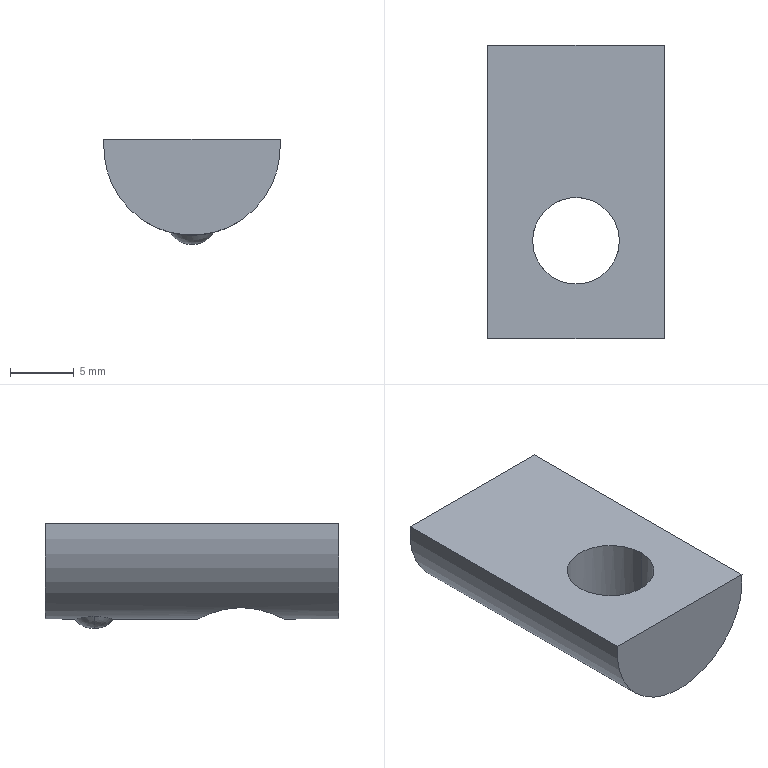Part | STEP file | HJLE-TXM-M8-40_LE0724153021 | 1 solid | 8 faces | box 13.848 x 23 x 8.25 mm | volume 1654 mm3 | cylinder 3 | plane 3 | spline 2 | commonest cylinder face diameters 6.8 x2 13.848 x1
STEP:
#1=CARTESIAN_POINT('',(1.711,11.5,-7.285));
#2=VERTEX_POINT('',#1);
#3=CARTESIAN_POINT('',(-1.711,11.5,-7.285));
#4=VERTEX_POINT('',#3);
#5=CARTESIAN_POINT('',(1.711,11.5,-7.285));
#6=CARTESIAN_POINT('',(1.711,11.609,-7.285));
#7=CARTESIAN_POINT('',(1.699,11.716,-7.288));
#8=CARTESIAN_POINT('',(1.652,11.925,-7.3));
#9=CARTESIAN_POINT('',(1.616,12.028,-7.309));
#10=CARTESIAN_POINT('',(1.479,12.318,-7.341));
#11=CARTESIAN_POINT('',(1.345,12.492,-7.37));
#12=CARTESIAN_POINT('',(1.104,12.701,-7.412));
#13=CARTESIAN_POINT('',(1.015,12.764,-7.426));
#14=CARTESIAN_POINT('',(0.83,12.872,-7.451));
#15=CARTESIAN_POINT('',(0.733,12.916,-7.462));
#16=CARTESIAN_POINT('',(0.5309,12.989,-7.48));
#17=CARTESIAN_POINT('',(0.4254,13.016,-7.488));
#18=CARTESIAN_POINT('',(0.2141,13.052,-7.497));
#19=CARTESIAN_POINT('',(0.1072,13.061,-7.5));
#20=CARTESIAN_POINT('',(-0.217,13.061,-7.5));
#21=CARTESIAN_POINT('',(-0.43,13.025,-7.49));
#22=CARTESIAN_POINT('',(-0.8362,12.879,-7.452));
#23=CARTESIAN_POINT('',(-1.022,12.773,-7.426));
#24=CARTESIAN_POINT('',(-1.347,12.49,-7.37));
#25=CARTESIAN_POINT('',(-1.478,12.32,-7.341));
#26=CARTESIAN_POINT('',(-1.616,12.028,-7.309));
#27=CARTESIAN_POINT('',(-1.651,11.927,-7.3));
#28=CARTESIAN_POINT('',(-1.699,11.718,-7.288));
#29=CARTESIAN_POINT('',(-1.711,11.609,-7.285));
#30=CARTESIAN_POINT('',(-1.711,11.5,-7.285));
#31=B_SPLINE_CURVE_WITH_KNOTS('',3,(#5,#6,#7,#8,#9,#10,#11,#12,#13,#14,#15,#16,#17,#18,#19,#20,#21,#22,#23,#24,#25,#26,#27,#28,#29,#30),.UNSPECIFIED.,.F.,.F.,(4,2,2,2,2,2,2,2,2,2,2,2,4),(0.,0.0003216,0.0006431,0.001286,0.001608,0.001929,0.002251,0.002573,0.003216,0.003859,0.004502,0.004824,0.005145),.UNSPECIFIED.);
#32=EDGE_CURVE('',#2,#4,#31,.T.);
#33=ORIENTED_EDGE('',*,*,#32,.F.);
#34=CARTESIAN_POINT('',(0.,11.5,-6.25));
#35=DIRECTION('',(0.,1.,0.));
#36=DIRECTION('',(1.,0.,0.));
#37=AXIS2_PLACEMENT_3D('',#34,#35,#36);
#38=CIRCLE('',#37,2.);
#39=EDGE_CURVE('',#2,#4,#38,.T.);
#40=ORIENTED_EDGE('',*,*,#39,.T.);
#41=EDGE_LOOP('',(#33,#40));
#42=FACE_OUTER_BOUND('',#41,.T.);
#43=CARTESIAN_POINT('',(1.724,11.5,-7.264));
#44=CARTESIAN_POINT('',(1.724,11.816,-7.264));
#45=CARTESIAN_POINT('',(1.724,12.1,-7.126));
#46=CARTESIAN_POINT('',(1.724,12.296,-6.879));
#47=CARTESIAN_POINT('',(0.8559,11.5,-8.74));
#48=CARTESIAN_POINT('',(0.8559,12.275,-8.74));
#49=CARTESIAN_POINT('',(0.8559,12.973,-8.402));
#50=CARTESIAN_POINT('',(0.8559,13.454,-7.793));
#51=CARTESIAN_POINT('',(-0.8559,11.5,-8.74));
#52=CARTESIAN_POINT('',(-0.8559,12.275,-8.74));
#53=CARTESIAN_POINT('',(-0.8559,12.973,-8.402));
#54=CARTESIAN_POINT('',(-0.8559,13.454,-7.793));
#55=CARTESIAN_POINT('',(-1.724,11.5,-7.264));
#56=CARTESIAN_POINT('',(-1.724,11.816,-7.264));
#57=CARTESIAN_POINT('',(-1.724,12.1,-7.126));
#58=CARTESIAN_POINT('',(-1.724,12.296,-6.879));
#59=(BOUNDED_SURFACE()B_SPLINE_SURFACE(3,3,((#43,#44,#45,#46),(#47,#48,#49,#50),(#51,#52,#53,#54),(#55,#56,#57,#58)),.UNSPECIFIED.,.F.,.F.,.T.)B_SPLINE_SURFACE_WITH_KNOTS((4,4),(4,4),(0.,1.),(0.,1.),.UNSPECIFIED.)GEOMETRIC_REPRESENTATION_ITEM()RATIONAL_B_SPLINE_SURFACE(((1.,0.9333,0.9333,1.),(0.6713,0.6266,0.6266,0.6713),(0.6713,0.6266,0.6266,0.6713),(1.,0.9333,0.9333,1.)))REPRESENTATION_ITEM('')SURFACE());
#60=ADVANCED_FACE('',(#42),#59,.T.);
#61=CARTESIAN_POINT('',(-3.4,0.,-6.608));
#62=VERTEX_POINT('',#61);
#63=CARTESIAN_POINT('',(3.4,0.,-6.608));
#64=VERTEX_POINT('',#63);
#65=CARTESIAN_POINT('',(-3.4,0.,-6.608));
#66=CARTESIAN_POINT('',(-3.4,-0.2286,-6.608));
#67=CARTESIAN_POINT('',(-3.377,-0.4525,-6.621));
#68=CARTESIAN_POINT('',(-3.289,-0.8916,-6.669));
#69=CARTESIAN_POINT('',(-3.222,-1.109,-6.706));
#70=CARTESIAN_POINT('',(-3.05,-1.518,-6.793));
#71=CARTESIAN_POINT('',(-2.946,-1.712,-6.843));
#72=CARTESIAN_POINT('',(-2.7,-2.078,-6.953));
#73=CARTESIAN_POINT('',(-2.56,-2.248,-7.011));
#74=CARTESIAN_POINT('',(-2.252,-2.557,-7.126));
#75=CARTESIAN_POINT('',(-2.082,-2.697,-7.182));
#76=CARTESIAN_POINT('',(-1.715,-2.944,-7.287));
#77=CARTESIAN_POINT('',(-1.521,-3.049,-7.334));
#78=CARTESIAN_POINT('',(-1.113,-3.22,-7.413));
#79=CARTESIAN_POINT('',(-0.8955,-3.288,-7.445));
#80=CARTESIAN_POINT('',(-0.4546,-3.377,-7.489));
#81=CARTESIAN_POINT('',(-0.2314,-3.4,-7.5));
#82=CARTESIAN_POINT('',(0.2211,-3.4,-7.5));
#83=CARTESIAN_POINT('',(0.4498,-3.378,-7.489));
#84=CARTESIAN_POINT('',(0.8899,-3.289,-7.446));
#85=CARTESIAN_POINT('',(1.106,-3.223,-7.414));
#86=CARTESIAN_POINT('',(1.519,-3.05,-7.335));
#87=CARTESIAN_POINT('',(1.713,-2.945,-7.287));
#88=CARTESIAN_POINT('',(2.079,-2.699,-7.183));
#89=CARTESIAN_POINT('',(2.251,-2.558,-7.126));
#90=CARTESIAN_POINT('',(2.559,-2.249,-7.012));
#91=CARTESIAN_POINT('',(2.698,-2.081,-6.954));
#92=CARTESIAN_POINT('',(2.945,-1.714,-6.844));
#93=CARTESIAN_POINT('',(3.05,-1.519,-6.793));
#94=CARTESIAN_POINT('',(3.22,-1.113,-6.706));
#95=CARTESIAN_POINT('',(3.287,-0.8987,-6.67));
#96=CARTESIAN_POINT('',(3.377,-0.4542,-6.621));
#97=CARTESIAN_POINT('',(3.4,-0.2285,-6.608));
#98=CARTESIAN_POINT('',(3.4,0.,-6.608));
#99=B_SPLINE_CURVE_WITH_KNOTS('',3,(#65,#66,#67,#68,#69,#70,#71,#72,#73,#74,#75,#76,#77,#78,#79,#80,#81,#82,#83,#84,#85,#86,#87,#88,#89,#90,#91,#92,#93,#94,#95,#96,#97,#98),.UNSPECIFIED.,.F.,.F.,(4,2,2,2,2,2,2,2,2,2,2,2,2,2,2,2,4),(0.0108,0.01148,0.01215,0.01282,0.0135,0.01417,0.01485,0.01552,0.0162,0.01687,0.01755,0.01822,0.0189,0.01957,0.02025,0.02092,0.0216),.UNSPECIFIED.);
#100=EDGE_CURVE('',#62,#64,#99,.T.);
#101=ORIENTED_EDGE('',*,*,#100,.F.);
#102=CARTESIAN_POINT('',(-3.4,0.,0.));
#103=VERTEX_POINT('',#102);
#104=CARTESIAN_POINT('',(-3.4,0.,0.));
#105=DIRECTION('',(0.,0.,1.));
#106=VECTOR('',#105,1000.);
#107=LINE('',#104,#106);
#108=EDGE_CURVE('',#62,#103,#107,.T.);
#109=ORIENTED_EDGE('',*,*,#108,.T.);
#110=CARTESIAN_POINT('',(3.4,0.,0.));
#111=VERTEX_POINT('',#110);
#112=CARTESIAN_POINT('',(0.,0.,0.));
#113=DIRECTION('',(0.,0.,-1.));
#114=DIRECTION('',(1.,0.,0.));
#115=AXIS2_PLACEMENT_3D('',#112,#113,#114);
#116=CIRCLE('',#115,3.4);
#117=EDGE_CURVE('',#111,#103,#116,.T.);
#118=ORIENTED_EDGE('',*,*,#117,.F.);
#119=CARTESIAN_POINT('',(3.4,0.,0.));
#120=DIRECTION('',(0.,0.,1.));
#121=VECTOR('',#120,1000.);
#122=LINE('',#119,#121);
#123=EDGE_CURVE('',#64,#111,#122,.T.);
#124=ORIENTED_EDGE('',*,*,#123,.F.);
#125=EDGE_LOOP('',(#101,#109,#118,#124));
#126=FACE_OUTER_BOUND('',#125,.T.);
#127=CARTESIAN_POINT('',(0.,0.,0.));
#128=DIRECTION('',(0.,0.,1.));
#129=DIRECTION('',(1.,0.,0.));
#130=AXIS2_PLACEMENT_3D('',#127,#128,#129);
#131=CYLINDRICAL_SURFACE('',#130,3.4);
#132=ADVANCED_FACE('',(#126),#131,.F.);
#133=CARTESIAN_POINT('',(6.9,15.333,0.));
#134=VERTEX_POINT('',#133);
#135=CARTESIAN_POINT('',(6.9,-7.667,0.));
#136=VERTEX_POINT('',#135);
#137=CARTESIAN_POINT('',(6.9,-7.667,0.));
#138=DIRECTION('',(0.,-1.,0.));
#139=VECTOR('',#138,1000.);
#140=LINE('',#137,#139);
#141=EDGE_CURVE('',#134,#136,#140,.T.);
#142=ORIENTED_EDGE('',*,*,#141,.T.);
#143=CARTESIAN_POINT('',(-6.9,-7.667,0.));
#144=VERTEX_POINT('',#143);
#145=CARTESIAN_POINT('',(0.,-7.667,-0.576));
#146=DIRECTION('',(0.,1.,0.));
#147=DIRECTION('',(0.,0.,1.));
#148=AXIS2_PLACEMENT_3D('',#145,#146,#147);
#149=CIRCLE('',#148,6.924);
#150=EDGE_CURVE('',#136,#144,#149,.T.);
#151=ORIENTED_EDGE('',*,*,#150,.T.);
#152=CARTESIAN_POINT('',(-6.9,15.333,0.));
#153=VERTEX_POINT('',#152);
#154=CARTESIAN_POINT('',(-6.9,-7.667,0.));
#155=DIRECTION('',(0.,1.,0.));
#156=VECTOR('',#155,1000.);
#157=LINE('',#154,#156);
#158=EDGE_CURVE('',#144,#153,#157,.T.);
#159=ORIENTED_EDGE('',*,*,#158,.T.);
#160=CARTESIAN_POINT('',(0.,15.333,-0.576));
#161=DIRECTION('',(0.,-1.,0.));
#162=DIRECTION('',(0.,0.,1.));
#163=AXIS2_PLACEMENT_3D('',#160,#161,#162);
#164=CIRCLE('',#163,6.924);
#165=EDGE_CURVE('',#153,#134,#164,.T.);
#166=ORIENTED_EDGE('',*,*,#165,.T.);
#167=EDGE_LOOP('',(#142,#151,#159,#166));
#168=FACE_OUTER_BOUND('',#167,.T.);
#169=ORIENTED_EDGE('',*,*,#32,.T.);
#170=CARTESIAN_POINT('',(-1.711,11.5,-7.285));
#171=CARTESIAN_POINT('',(-1.711,11.391,-7.285));
#172=CARTESIAN_POINT('',(-1.699,11.284,-7.288));
#173=CARTESIAN_POINT('',(-1.652,11.075,-7.3));
#174=CARTESIAN_POINT('',(-1.616,10.972,-7.309));
#175=CARTESIAN_POINT('',(-1.479,10.682,-7.341));
#176=CARTESIAN_POINT('',(-1.345,10.508,-7.37));
#177=CARTESIAN_POINT('',(-1.104,10.299,-7.412));
#178=CARTESIAN_POINT('',(-1.015,10.236,-7.426));
#179=CARTESIAN_POINT('',(-0.83,10.128,-7.451));
#180=CARTESIAN_POINT('',(-0.733,10.084,-7.462));
#181=CARTESIAN_POINT('',(-0.5309,10.011,-7.48));
#182=CARTESIAN_POINT('',(-0.4254,9.984,-7.488));
#183=CARTESIAN_POINT('',(-0.2141,9.948,-7.497));
#184=CARTESIAN_POINT('',(-0.1072,9.939,-7.5));
#185=CARTESIAN_POINT('',(0.217,9.939,-7.5));
#186=CARTESIAN_POINT('',(0.43,9.975,-7.49));
#187=CARTESIAN_POINT('',(0.8362,10.121,-7.452));
#188=CARTESIAN_POINT('',(1.022,10.227,-7.426));
#189=CARTESIAN_POINT('',(1.347,10.51,-7.37));
#190=CARTESIAN_POINT('',(1.478,10.68,-7.341));
#191=CARTESIAN_POINT('',(1.616,10.972,-7.309));
#192=CARTESIAN_POINT('',(1.651,11.073,-7.3));
#193=CARTESIAN_POINT('',(1.699,11.282,-7.288));
#194=CARTESIAN_POINT('',(1.711,11.391,-7.285));
#195=CARTESIAN_POINT('',(1.711,11.5,-7.285));
#196=B_SPLINE_CURVE_WITH_KNOTS('',3,(#170,#171,#172,#173,#174,#175,#176,#177,#178,#179,#180,#181,#182,#183,#184,#185,#186,#187,#188,#189,#190,#191,#192,#193,#194,#195),.UNSPECIFIED.,.F.,.F.,(4,2,2,2,2,2,2,2,2,2,2,2,4),(0.005145,0.005466,0.005788,0.006431,0.006752,0.007073,0.007395,0.007716,0.008359,0.009002,0.009644,0.009966,0.01029),.UNSPECIFIED.);
#197=EDGE_CURVE('',#4,#2,#196,.T.);
#198=ORIENTED_EDGE('',*,*,#197,.T.);
#199=EDGE_LOOP('',(#169,#198));
#200=FACE_BOUND('',#199,.T.);
#201=CARTESIAN_POINT('',(3.4,0.,-6.608));
#202=CARTESIAN_POINT('',(3.4,0.2286,-6.608));
#203=CARTESIAN_POINT('',(3.377,0.4525,-6.621));
#204=CARTESIAN_POINT('',(3.289,0.8916,-6.669));
#205=CARTESIAN_POINT('',(3.222,1.109,-6.706));
#206=CARTESIAN_POINT('',(3.05,1.518,-6.793));
#207=CARTESIAN_POINT('',(2.946,1.712,-6.843));
#208=CARTESIAN_POINT('',(2.7,2.078,-6.953));
#209=CARTESIAN_POINT('',(2.56,2.248,-7.011));
#210=CARTESIAN_POINT('',(2.252,2.557,-7.126));
#211=CARTESIAN_POINT('',(2.082,2.697,-7.182));
#212=CARTESIAN_POINT('',(1.715,2.944,-7.287));
#213=CARTESIAN_POINT('',(1.521,3.049,-7.334));
#214=CARTESIAN_POINT('',(1.113,3.22,-7.413));
#215=CARTESIAN_POINT('',(0.8955,3.288,-7.445));
#216=CARTESIAN_POINT('',(0.4546,3.377,-7.489));
#217=CARTESIAN_POINT('',(0.2314,3.4,-7.5));
#218=CARTESIAN_POINT('',(-0.2211,3.4,-7.5));
#219=CARTESIAN_POINT('',(-0.4498,3.378,-7.489));
#220=CARTESIAN_POINT('',(-0.8899,3.289,-7.446));
#221=CARTESIAN_POINT('',(-1.106,3.223,-7.414));
#222=CARTESIAN_POINT('',(-1.519,3.05,-7.335));
#223=CARTESIAN_POINT('',(-1.713,2.945,-7.287));
#224=CARTESIAN_POINT('',(-2.079,2.699,-7.183));
#225=CARTESIAN_POINT('',(-2.251,2.558,-7.126));
#226=CARTESIAN_POINT('',(-2.559,2.249,-7.012));
#227=CARTESIAN_POINT('',(-2.698,2.081,-6.954));
#228=CARTESIAN_POINT('',(-2.945,1.714,-6.844));
#229=CARTESIAN_POINT('',(-3.05,1.519,-6.793));
#230=CARTESIAN_POINT('',(-3.22,1.113,-6.706));
#231=CARTESIAN_POINT('',(-3.287,0.8987,-6.67));
#232=CARTESIAN_POINT('',(-3.377,0.4542,-6.621));
#233=CARTESIAN_POINT('',(-3.4,0.2288,-6.608));
#234=CARTESIAN_POINT('',(-3.4,0.,-6.608));
#235=B_SPLINE_CURVE_WITH_KNOTS('',3,(#201,#202,#203,#204,#205,#206,#207,#208,#209,#210,#211,#212,#213,#214,#215,#216,#217,#218,#219,#220,#221,#222,#223,#224,#225,#226,#227,#228,#229,#230,#231,#232,#233,#234),.UNSPECIFIED.,.F.,.F.,(4,2,2,2,2,2,2,2,2,2,2,2,2,2,2,2,4),(0.,0.0006751,0.00135,0.002025,0.0027,0.003375,0.00405,0.004725,0.0054,0.006075,0.006751,0.007426,0.008101,0.008776,0.009451,0.01013,0.0108),.UNSPECIFIED.);
#236=EDGE_CURVE('',#64,#62,#235,.T.);
#237=ORIENTED_EDGE('',*,*,#236,.T.);
#238=ORIENTED_EDGE('',*,*,#100,.T.);
#239=EDGE_LOOP('',(#237,#238));
#240=FACE_BOUND('',#239,.T.);
#241=CARTESIAN_POINT('',(0.,-7.667,-0.576));
#242=DIRECTION('',(0.,1.,0.));
#243=DIRECTION('',(0.,0.,1.));
#244=AXIS2_PLACEMENT_3D('',#241,#242,#243);
#245=CYLINDRICAL_SURFACE('',#244,6.924);
#246=ADVANCED_FACE('',(#168,#200,#240),#245,.T.);
#247=CARTESIAN_POINT('',(0.,-7.667,0.));
#248=DIRECTION('',(-1.,0.,0.));
#249=VECTOR('',#248,1000.);
#250=LINE('',#247,#249);
#251=EDGE_CURVE('',#136,#144,#250,.T.);
#252=ORIENTED_EDGE('',*,*,#251,.T.);
#253=ORIENTED_EDGE('',*,*,#150,.F.);
#254=EDGE_LOOP('',(#252,#253));
#255=FACE_OUTER_BOUND('',#254,.T.);
#256=CARTESIAN_POINT('',(0.,-7.667,-0.576));
#257=DIRECTION('',(0.,-1.,0.));
#258=DIRECTION('',(0.,0.,-1.));
#259=AXIS2_PLACEMENT_3D('',#256,#257,#258);
#260=PLANE('',#259);
#261=ADVANCED_FACE('',(#255),#260,.T.);
#262=ORIENTED_EDGE('',*,*,#158,.F.);
#263=ORIENTED_EDGE('',*,*,#251,.F.);
#264=ORIENTED_EDGE('',*,*,#141,.F.);
#265=CARTESIAN_POINT('',(0.,15.333,0.));
#266=DIRECTION('',(-1.,0.,0.));
#267=VECTOR('',#266,1000.);
#268=LINE('',#265,#267);
#269=EDGE_CURVE('',#134,#153,#268,.T.);
#270=ORIENTED_EDGE('',*,*,#269,.T.);
#271=EDGE_LOOP('',(#262,#263,#264,#270));
#272=FACE_OUTER_BOUND('',#271,.T.);
#273=ORIENTED_EDGE('',*,*,#117,.T.);
#274=CARTESIAN_POINT('',(0.,0.,0.));
#275=DIRECTION('',(0.,0.,-1.));
#276=DIRECTION('',(1.,0.,0.));
#277=AXIS2_PLACEMENT_3D('',#274,#275,#276);
#278=CIRCLE('',#277,3.4);
#279=EDGE_CURVE('',#103,#111,#278,.T.);
#280=ORIENTED_EDGE('',*,*,#279,.T.);
#281=EDGE_LOOP('',(#273,#280));
#282=FACE_BOUND('',#281,.T.);
#283=CARTESIAN_POINT('',(0.,-7.667,0.));
#284=DIRECTION('',(0.,0.,1.));
#285=DIRECTION('',(1.,0.,0.));
#286=AXIS2_PLACEMENT_3D('',#283,#284,#285);
#287=PLANE('',#286);
#288=ADVANCED_FACE('',(#272,#282),#287,.T.);
#289=ORIENTED_EDGE('',*,*,#165,.F.);
#290=ORIENTED_EDGE('',*,*,#269,.F.);
#291=EDGE_LOOP('',(#289,#290));
#292=FACE_OUTER_BOUND('',#291,.T.);
#293=CARTESIAN_POINT('',(0.,15.333,-0.576));
#294=DIRECTION('',(0.,-1.,0.));
#295=DIRECTION('',(0.,0.,-1.));
#296=AXIS2_PLACEMENT_3D('',#293,#294,#295);
#297=PLANE('',#296);
#298=ADVANCED_FACE('',(#292),#297,.F.);
#299=ORIENTED_EDGE('',*,*,#39,.F.);
#300=ORIENTED_EDGE('',*,*,#197,.F.);
#301=EDGE_LOOP('',(#299,#300));
#302=FACE_OUTER_BOUND('',#301,.T.);
#303=CARTESIAN_POINT('',(1.724,10.704,-6.879));
#304=CARTESIAN_POINT('',(1.724,10.9,-7.126));
#305=CARTESIAN_POINT('',(1.724,11.184,-7.264));
#306=CARTESIAN_POINT('',(1.724,11.5,-7.264));
#307=CARTESIAN_POINT('',(0.8559,9.546,-7.793));
#308=CARTESIAN_POINT('',(0.8559,10.027,-8.402));
#309=CARTESIAN_POINT('',(0.8559,10.725,-8.74));
#310=CARTESIAN_POINT('',(0.8559,11.5,-8.74));
#311=CARTESIAN_POINT('',(-0.8559,9.546,-7.793));
#312=CARTESIAN_POINT('',(-0.8559,10.027,-8.402));
#313=CARTESIAN_POINT('',(-0.8559,10.725,-8.74));
#314=CARTESIAN_POINT('',(-0.8559,11.5,-8.74));
#315=CARTESIAN_POINT('',(-1.724,10.704,-6.879));
#316=CARTESIAN_POINT('',(-1.724,10.9,-7.126));
#317=CARTESIAN_POINT('',(-1.724,11.184,-7.264));
#318=CARTESIAN_POINT('',(-1.724,11.5,-7.264));
#319=(BOUNDED_SURFACE()B_SPLINE_SURFACE(3,3,((#303,#304,#305,#306),(#307,#308,#309,#310),(#311,#312,#313,#314),(#315,#316,#317,#318)),.UNSPECIFIED.,.F.,.F.,.T.)B_SPLINE_SURFACE_WITH_KNOTS((4,4),(4,4),(0.,1.),(0.,1.),.UNSPECIFIED.)GEOMETRIC_REPRESENTATION_ITEM()RATIONAL_B_SPLINE_SURFACE(((1.,0.9333,0.9333,1.),(0.6713,0.6266,0.6266,0.6713),(0.6713,0.6266,0.6266,0.6713),(1.,0.9333,0.9333,1.)))REPRESENTATION_ITEM('')SURFACE());
#320=ADVANCED_FACE('',(#302),#319,.T.);
#321=ORIENTED_EDGE('',*,*,#108,.F.);
#322=ORIENTED_EDGE('',*,*,#236,.F.);
#323=ORIENTED_EDGE('',*,*,#123,.T.);
#324=ORIENTED_EDGE('',*,*,#279,.F.);
#325=EDGE_LOOP('',(#321,#322,#323,#324));
#326=FACE_OUTER_BOUND('',#325,.T.);
#327=CARTESIAN_POINT('',(0.,0.,0.));
#328=DIRECTION('',(0.,0.,1.));
#329=DIRECTION('',(1.,0.,0.));
#330=AXIS2_PLACEMENT_3D('',#327,#328,#329);
#331=CYLINDRICAL_SURFACE('',#330,3.4);
#332=ADVANCED_FACE('',(#326),#331,.F.);
#333=CLOSED_SHELL('',(#60,#132,#246,#261,#288,#298,#320,#332));
#334=MANIFOLD_SOLID_BREP('',#333);
#335=CARTESIAN_POINT('',(0.,0.,0.));
#336=DIRECTION('',(0.,0.,1.));
#337=DIRECTION('',(1.,0.,0.));
#338=AXIS2_PLACEMENT_3D('',#335,#336,#337);
#339=(LENGTH_UNIT()NAMED_UNIT(*)SI_UNIT(.MILLI.,.METRE.));
#340=UNCERTAINTY_MEASURE_WITH_UNIT(LENGTH_MEASURE(0.00001),#339,'','');
#341=(NAMED_UNIT(*)PLANE_ANGLE_UNIT()SI_UNIT($,.RADIAN.));
#342=(NAMED_UNIT(*)SI_UNIT($,.STERADIAN.)SOLID_ANGLE_UNIT());
#343=(GEOMETRIC_REPRESENTATION_CONTEXT(3)GLOBAL_UNCERTAINTY_ASSIGNED_CONTEXT((#340))GLOBAL_UNIT_ASSIGNED_CONTEXT((#339,#341,#342))REPRESENTATION_CONTEXT('',''));
#344=ADVANCED_BREP_SHAPE_REPRESENTATION('',(#334,#338),#343);